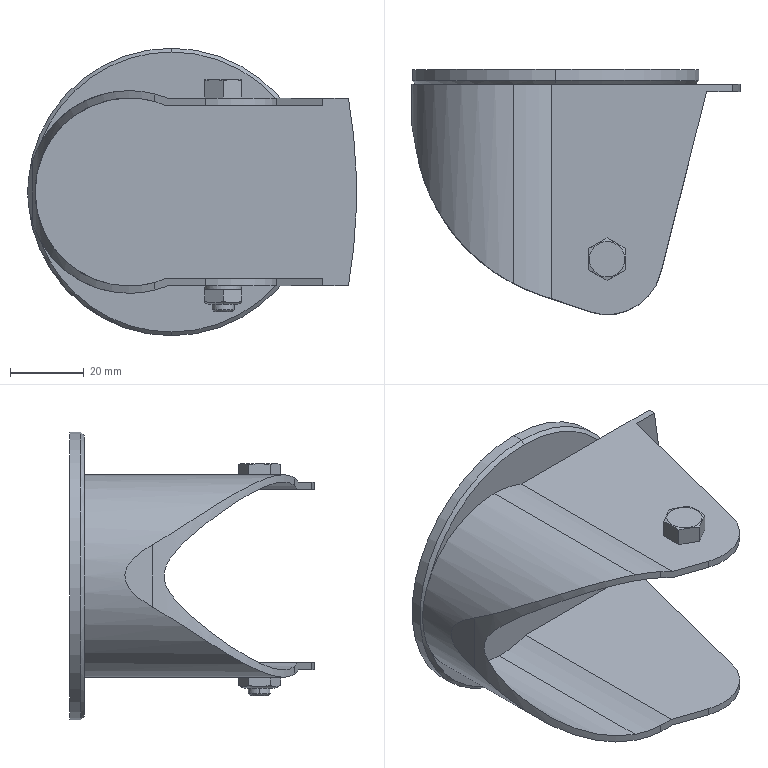Part | SolidWorks | features BaseBody 1 | 1 solid | 59 faces | box 89.183 x 66.5 x 78 mm | volume 44639 mm3 | plane 35 | cylinder 16 | cone 6 | torus 2 | commonest cylinder face diameters 51 x3 55 x3 6 x2 10 x2 30 x2 78 x2